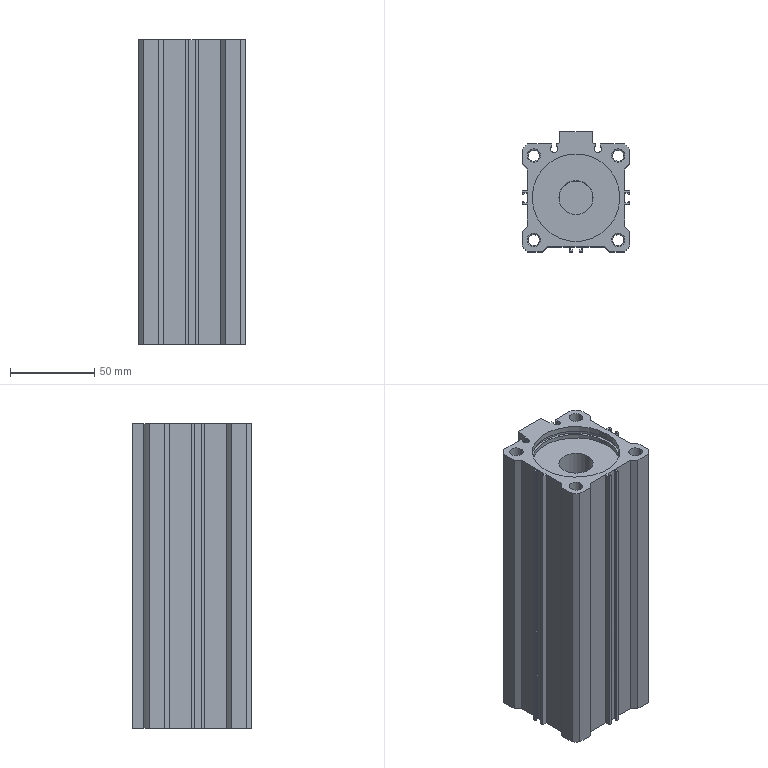Part | STEP file | CQ2A50-125DC-R06US_CQ2Tube | 1 solid | 156 faces | box 64 x 71 x 180.5 mm | volume 380542 mm3 | plane 74 | cylinder 54 | cone 28 | commonest cylinder face diameters 8 x16 6.6 x8 4.15 x6 10.7 x4 20.25 x4 52 x4